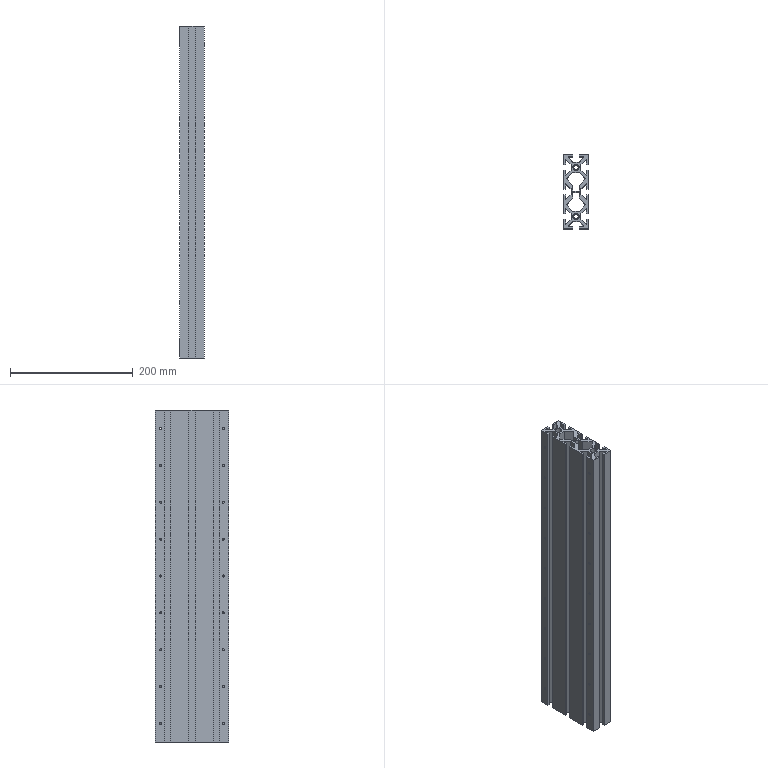Part | 1 solid | 186 faces | box 40 x 120 x 540 mm | volume 1120992 mm3 | plane 90 | cylinder 88 | cone 8 | commonest cylinder face diameters 3.3 x72 10.2 x8 3 x4 6.8 x4